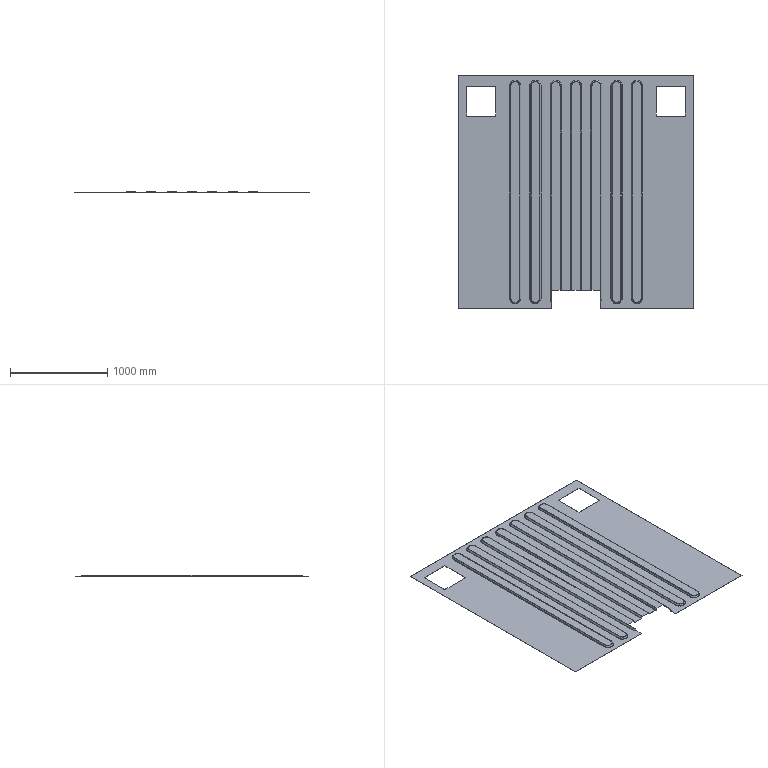Part | STEP file | 750038168 | 1 solid | 205 faces | box 2428 x 2404 x 19.9 mm | volume 8825097 mm3 | plane 62 | spline 58 | cylinder 56 | cone 29 | commonest cylinder face diameters 4 x28 7 x28